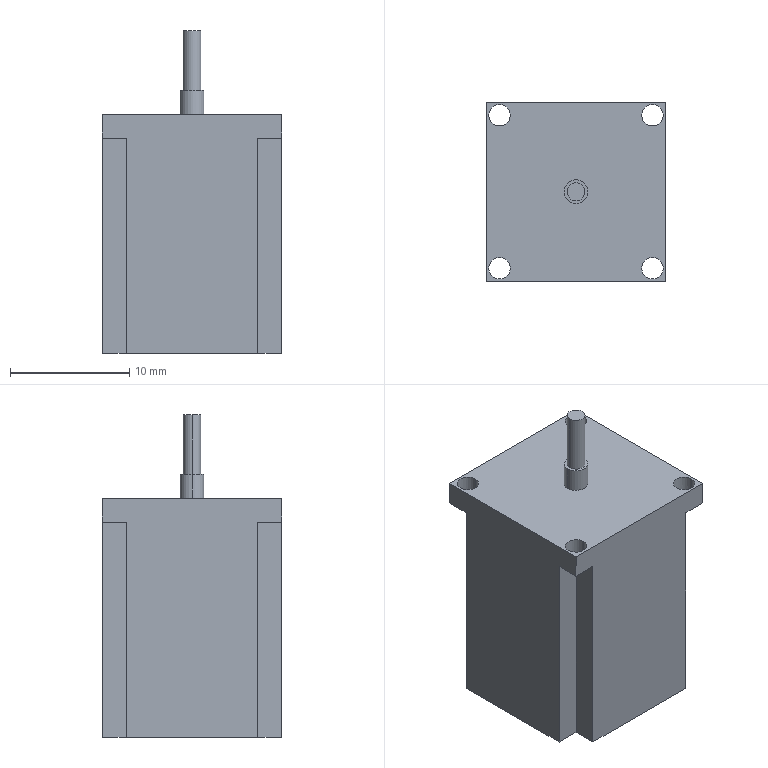Part | SolidWorks | features ICE 4, Extrusion 1 | 1 solid | 36 faces | box 15 x 15 x 27 mm | volume 4207 mm3 | plane 24 | cylinder 12 | commonest cylinder face diameters 1.8 x8 1.5 x2 2 x2
STEP:
#1=CARTESIAN_POINT('',(0.75,0.,27.));
#2=VERTEX_POINT('',#1);
#3=CARTESIAN_POINT('',(-0.75,0.,27.));
#4=VERTEX_POINT('',#3);
#5=CARTESIAN_POINT('',(0.,0.,27.));
#6=DIRECTION('',(0.,0.,1.));
#7=DIRECTION('',(1.,0.,0.));
#8=AXIS2_PLACEMENT_3D('',#5,#6,#7);
#9=CIRCLE('',#8,0.75);
#10=EDGE_CURVE('',#2,#4,#9,.T.);
#11=ORIENTED_EDGE('',*,*,#10,.F.);
#12=CARTESIAN_POINT('',(0.75,0.,22.));
#13=VERTEX_POINT('',#12);
#14=CARTESIAN_POINT('',(0.75,0.,27.));
#15=DIRECTION('',(0.,0.,-1.));
#16=VECTOR('',#15,1000.);
#17=LINE('',#14,#16);
#18=EDGE_CURVE('',#2,#13,#17,.T.);
#19=ORIENTED_EDGE('',*,*,#18,.T.);
#20=CARTESIAN_POINT('',(-0.75,0.,22.));
#21=VERTEX_POINT('',#20);
#22=CARTESIAN_POINT('',(0.,0.,22.));
#23=DIRECTION('',(0.,0.,1.));
#24=DIRECTION('',(1.,0.,0.));
#25=AXIS2_PLACEMENT_3D('',#22,#23,#24);
#26=CIRCLE('',#25,0.75);
#27=EDGE_CURVE('',#13,#21,#26,.T.);
#28=ORIENTED_EDGE('',*,*,#27,.T.);
#29=CARTESIAN_POINT('',(-0.75,0.,27.));
#30=DIRECTION('',(0.,0.,-1.));
#31=VECTOR('',#30,1000.);
#32=LINE('',#29,#31);
#33=EDGE_CURVE('',#4,#21,#32,.T.);
#34=ORIENTED_EDGE('',*,*,#33,.F.);
#35=EDGE_LOOP('',(#11,#19,#28,#34));
#36=FACE_OUTER_BOUND('',#35,.T.);
#37=CARTESIAN_POINT('',(0.,0.,27.));
#38=DIRECTION('',(0.,0.,-1.));
#39=DIRECTION('',(-1.,0.,0.));
#40=AXIS2_PLACEMENT_3D('',#37,#38,#39);
#41=CYLINDRICAL_SURFACE('',#40,0.75);
#42=ADVANCED_FACE('',(#36),#41,.T.);
#43=CARTESIAN_POINT('',(1.,0.,22.));
#44=VERTEX_POINT('',#43);
#45=CARTESIAN_POINT('',(-1.,0.,22.));
#46=VERTEX_POINT('',#45);
#47=CARTESIAN_POINT('',(0.,0.,22.));
#48=DIRECTION('',(0.,0.,1.));
#49=DIRECTION('',(1.,0.,0.));
#50=AXIS2_PLACEMENT_3D('',#47,#48,#49);
#51=CIRCLE('',#50,1.);
#52=EDGE_CURVE('',#44,#46,#51,.T.);
#53=ORIENTED_EDGE('',*,*,#52,.F.);
#54=CARTESIAN_POINT('',(1.,0.,20.));
#55=VERTEX_POINT('',#54);
#56=CARTESIAN_POINT('',(1.,0.,22.));
#57=DIRECTION('',(0.,0.,-1.));
#58=VECTOR('',#57,1000.);
#59=LINE('',#56,#58);
#60=EDGE_CURVE('',#44,#55,#59,.T.);
#61=ORIENTED_EDGE('',*,*,#60,.T.);
#62=CARTESIAN_POINT('',(-1.,0.,20.));
#63=VERTEX_POINT('',#62);
#64=CARTESIAN_POINT('',(0.,0.,20.));
#65=DIRECTION('',(0.,0.,1.));
#66=DIRECTION('',(-1.,0.,0.));
#67=AXIS2_PLACEMENT_3D('',#64,#65,#66);
#68=CIRCLE('',#67,1.);
#69=EDGE_CURVE('',#55,#63,#68,.T.);
#70=ORIENTED_EDGE('',*,*,#69,.T.);
#71=CARTESIAN_POINT('',(-1.,0.,22.));
#72=DIRECTION('',(0.,0.,-1.));
#73=VECTOR('',#72,1000.);
#74=LINE('',#71,#73);
#75=EDGE_CURVE('',#46,#63,#74,.T.);
#76=ORIENTED_EDGE('',*,*,#75,.F.);
#77=EDGE_LOOP('',(#53,#61,#70,#76));
#78=FACE_OUTER_BOUND('',#77,.T.);
#79=CARTESIAN_POINT('',(0.,0.,22.));
#80=DIRECTION('',(0.,0.,-1.));
#81=DIRECTION('',(-1.,0.,0.));
#82=AXIS2_PLACEMENT_3D('',#79,#80,#81);
#83=CYLINDRICAL_SURFACE('',#82,1.);
#84=ADVANCED_FACE('',(#78),#83,.T.);
#85=CARTESIAN_POINT('',(-7.3,6.4,18.));
#86=VERTEX_POINT('',#85);
#87=CARTESIAN_POINT('',(-6.4,5.5,18.));
#88=VERTEX_POINT('',#87);
#89=CARTESIAN_POINT('',(-6.4,6.4,18.));
#90=DIRECTION('',(0.,0.,1.));
#91=DIRECTION('',(1.,0.,0.));
#92=AXIS2_PLACEMENT_3D('',#89,#90,#91);
#93=CIRCLE('',#92,0.9);
#94=EDGE_CURVE('',#86,#88,#93,.T.);
#95=ORIENTED_EDGE('',*,*,#94,.F.);
#96=CARTESIAN_POINT('',(-7.3,6.4,20.));
#97=VERTEX_POINT('',#96);
#98=CARTESIAN_POINT('',(-7.3,6.4,-51.));
#99=DIRECTION('',(0.,0.,1.));
#100=VECTOR('',#99,1000.);
#101=LINE('',#98,#100);
#102=EDGE_CURVE('',#86,#97,#101,.T.);
#103=ORIENTED_EDGE('',*,*,#102,.T.);
#104=CARTESIAN_POINT('',(-5.5,6.4,20.));
#105=VERTEX_POINT('',#104);
#106=CARTESIAN_POINT('',(-6.4,6.4,20.));
#107=DIRECTION('',(0.,0.,1.));
#108=DIRECTION('',(1.,0.,0.));
#109=AXIS2_PLACEMENT_3D('',#106,#107,#108);
#110=CIRCLE('',#109,0.9);
#111=EDGE_CURVE('',#97,#105,#110,.T.);
#112=ORIENTED_EDGE('',*,*,#111,.T.);
#113=CARTESIAN_POINT('',(-5.5,6.4,18.));
#114=VERTEX_POINT('',#113);
#115=CARTESIAN_POINT('',(-5.5,6.4,-51.));
#116=DIRECTION('',(0.,0.,1.));
#117=VECTOR('',#116,1000.);
#118=LINE('',#115,#117);
#119=EDGE_CURVE('',#114,#105,#118,.T.);
#120=ORIENTED_EDGE('',*,*,#119,.F.);
#121=CARTESIAN_POINT('',(-6.4,6.4,18.));
#122=DIRECTION('',(0.,0.,1.));
#123=DIRECTION('',(1.,0.,0.));
#124=AXIS2_PLACEMENT_3D('',#121,#122,#123);
#125=CIRCLE('',#124,0.9);
#126=EDGE_CURVE('',#88,#114,#125,.T.);
#127=ORIENTED_EDGE('',*,*,#126,.F.);
#128=EDGE_LOOP('',(#95,#103,#112,#120,#127));
#129=FACE_OUTER_BOUND('',#128,.T.);
#130=CARTESIAN_POINT('',(-6.4,6.4,-51.));
#131=DIRECTION('',(0.,0.,1.));
#132=DIRECTION('',(1.,0.,0.));
#133=AXIS2_PLACEMENT_3D('',#130,#131,#132);
#134=CYLINDRICAL_SURFACE('',#133,0.9);
#135=ADVANCED_FACE('',(#129),#134,.F.);
#136=CARTESIAN_POINT('',(5.5,-6.4,18.));
#137=VERTEX_POINT('',#136);
#138=CARTESIAN_POINT('',(7.3,-6.4,18.));
#139=VERTEX_POINT('',#138);
#140=CARTESIAN_POINT('',(6.4,-6.4,18.));
#141=DIRECTION('',(0.,0.,1.));
#142=DIRECTION('',(1.,0.,0.));
#143=AXIS2_PLACEMENT_3D('',#140,#141,#142);
#144=CIRCLE('',#143,0.9);
#145=EDGE_CURVE('',#137,#139,#144,.T.);
#146=ORIENTED_EDGE('',*,*,#145,.F.);
#147=CARTESIAN_POINT('',(5.5,-6.4,20.));
#148=VERTEX_POINT('',#147);
#149=CARTESIAN_POINT('',(5.5,-6.4,-51.));
#150=DIRECTION('',(0.,0.,1.));
#151=VECTOR('',#150,1000.);
#152=LINE('',#149,#151);
#153=EDGE_CURVE('',#137,#148,#152,.T.);
#154=ORIENTED_EDGE('',*,*,#153,.T.);
#155=CARTESIAN_POINT('',(7.3,-6.4,20.));
#156=VERTEX_POINT('',#155);
#157=CARTESIAN_POINT('',(6.4,-6.4,20.));
#158=DIRECTION('',(0.,0.,1.));
#159=DIRECTION('',(1.,0.,0.));
#160=AXIS2_PLACEMENT_3D('',#157,#158,#159);
#161=CIRCLE('',#160,0.9);
#162=EDGE_CURVE('',#148,#156,#161,.T.);
#163=ORIENTED_EDGE('',*,*,#162,.T.);
#164=CARTESIAN_POINT('',(7.3,-6.4,-51.));
#165=DIRECTION('',(0.,0.,1.));
#166=VECTOR('',#165,1000.);
#167=LINE('',#164,#166);
#168=EDGE_CURVE('',#139,#156,#167,.T.);
#169=ORIENTED_EDGE('',*,*,#168,.F.);
#170=EDGE_LOOP('',(#146,#154,#163,#169));
#171=FACE_OUTER_BOUND('',#170,.T.);
#172=CARTESIAN_POINT('',(6.4,-6.4,-51.));
#173=DIRECTION('',(0.,0.,1.));
#174=DIRECTION('',(1.,0.,0.));
#175=AXIS2_PLACEMENT_3D('',#172,#173,#174);
#176=CYLINDRICAL_SURFACE('',#175,0.9);
#177=ADVANCED_FACE('',(#171),#176,.F.);
#178=CARTESIAN_POINT('',(-5.5,-6.4,18.));
#179=VERTEX_POINT('',#178);
#180=CARTESIAN_POINT('',(-7.3,-6.4,18.));
#181=VERTEX_POINT('',#180);
#182=CARTESIAN_POINT('',(-6.4,-6.4,18.));
#183=DIRECTION('',(0.,0.,-1.));
#184=DIRECTION('',(-1.,0.,0.));
#185=AXIS2_PLACEMENT_3D('',#182,#183,#184);
#186=CIRCLE('',#185,0.9);
#187=EDGE_CURVE('',#179,#181,#186,.T.);
#188=ORIENTED_EDGE('',*,*,#187,.T.);
#189=CARTESIAN_POINT('',(-7.3,-6.4,20.));
#190=VERTEX_POINT('',#189);
#191=CARTESIAN_POINT('',(-7.3,-6.4,-51.));
#192=DIRECTION('',(0.,0.,1.));
#193=VECTOR('',#192,1000.);
#194=LINE('',#191,#193);
#195=EDGE_CURVE('',#181,#190,#194,.T.);
#196=ORIENTED_EDGE('',*,*,#195,.T.);
#197=CARTESIAN_POINT('',(-5.5,-6.4,20.));
#198=VERTEX_POINT('',#197);
#199=CARTESIAN_POINT('',(-6.4,-6.4,20.));
#200=DIRECTION('',(0.,0.,1.));
#201=DIRECTION('',(1.,0.,0.));
#202=AXIS2_PLACEMENT_3D('',#199,#200,#201);
#203=CIRCLE('',#202,0.9);
#204=EDGE_CURVE('',#190,#198,#203,.T.);
#205=ORIENTED_EDGE('',*,*,#204,.T.);
#206=CARTESIAN_POINT('',(-5.5,-6.4,-51.));
#207=DIRECTION('',(0.,0.,1.));
#208=VECTOR('',#207,1000.);
#209=LINE('',#206,#208);
#210=EDGE_CURVE('',#179,#198,#209,.T.);
#211=ORIENTED_EDGE('',*,*,#210,.F.);
#212=EDGE_LOOP('',(#188,#196,#205,#211));
#213=FACE_OUTER_BOUND('',#212,.T.);
#214=CARTESIAN_POINT('',(-6.4,-6.4,-51.));
#215=DIRECTION('',(0.,0.,1.));
#216=DIRECTION('',(1.,0.,0.));
#217=AXIS2_PLACEMENT_3D('',#214,#215,#216);
#218=CYLINDRICAL_SURFACE('',#217,0.9);
#219=ADVANCED_FACE('',(#213),#218,.F.);
#220=CARTESIAN_POINT('',(6.4,5.5,18.));
#221=VERTEX_POINT('',#220);
#222=CARTESIAN_POINT('',(5.5,6.4,18.));
#223=VERTEX_POINT('',#222);
#224=CARTESIAN_POINT('',(6.4,6.4,18.));
#225=DIRECTION('',(0.,0.,-1.));
#226=DIRECTION('',(-1.,0.,0.));
#227=AXIS2_PLACEMENT_3D('',#224,#225,#226);
#228=CIRCLE('',#227,0.9);
#229=EDGE_CURVE('',#221,#223,#228,.T.);
#230=ORIENTED_EDGE('',*,*,#229,.T.);
#231=CARTESIAN_POINT('',(5.5,6.4,20.));
#232=VERTEX_POINT('',#231);
#233=CARTESIAN_POINT('',(5.5,6.4,-51.));
#234=DIRECTION('',(0.,0.,1.));
#235=VECTOR('',#234,1000.);
#236=LINE('',#233,#235);
#237=EDGE_CURVE('',#223,#232,#236,.T.);
#238=ORIENTED_EDGE('',*,*,#237,.T.);
#239=CARTESIAN_POINT('',(7.3,6.4,20.));
#240=VERTEX_POINT('',#239);
#241=CARTESIAN_POINT('',(6.4,6.4,20.));
#242=DIRECTION('',(0.,0.,1.));
#243=DIRECTION('',(1.,0.,0.));
#244=AXIS2_PLACEMENT_3D('',#241,#242,#243);
#245=CIRCLE('',#244,0.9);
#246=EDGE_CURVE('',#232,#240,#245,.T.);
#247=ORIENTED_EDGE('',*,*,#246,.T.);
#248=CARTESIAN_POINT('',(7.3,6.4,18.));
#249=VERTEX_POINT('',#248);
#250=CARTESIAN_POINT('',(7.3,6.4,-51.));
#251=DIRECTION('',(0.,0.,1.));
#252=VECTOR('',#251,1000.);
#253=LINE('',#250,#252);
#254=EDGE_CURVE('',#249,#240,#253,.T.);
#255=ORIENTED_EDGE('',*,*,#254,.F.);
#256=CARTESIAN_POINT('',(6.4,6.4,18.));
#257=DIRECTION('',(0.,0.,-1.));
#258=DIRECTION('',(-1.,0.,0.));
#259=AXIS2_PLACEMENT_3D('',#256,#257,#258);
#260=CIRCLE('',#259,0.9);
#261=EDGE_CURVE('',#249,#221,#260,.T.);
#262=ORIENTED_EDGE('',*,*,#261,.T.);
#263=EDGE_LOOP('',(#230,#238,#247,#255,#262));
#264=FACE_OUTER_BOUND('',#263,.T.);
#265=CARTESIAN_POINT('',(6.4,6.4,-51.));
#266=DIRECTION('',(0.,0.,1.));
#267=DIRECTION('',(1.,0.,0.));
#268=AXIS2_PLACEMENT_3D('',#265,#266,#267);
#269=CYLINDRICAL_SURFACE('',#268,0.9);
#270=ADVANCED_FACE('',(#264),#269,.F.);
#271=CARTESIAN_POINT('',(-5.5,7.5,18.));
#272=VERTEX_POINT('',#271);
#273=CARTESIAN_POINT('',(-5.5,7.5,18.));
#274=DIRECTION('',(0.,-1.,0.));
#275=VECTOR('',#274,1000.);
#276=LINE('',#273,#275);
#277=EDGE_CURVE('',#272,#114,#276,.T.);
#278=ORIENTED_EDGE('',*,*,#277,.T.);
#279=CARTESIAN_POINT('',(-6.4,6.4,18.));
#280=DIRECTION('',(0.,0.,1.));
#281=DIRECTION('',(1.,0.,0.));
#282=AXIS2_PLACEMENT_3D('',#279,#280,#281);
#283=CIRCLE('',#282,0.9);
#284=EDGE_CURVE('',#114,#86,#283,.T.);
#285=ORIENTED_EDGE('',*,*,#284,.T.);
#286=ORIENTED_EDGE('',*,*,#94,.T.);
#287=CARTESIAN_POINT('',(-7.5,5.5,18.));
#288=VERTEX_POINT('',#287);
#289=CARTESIAN_POINT('',(-7.5,5.5,18.));
#290=DIRECTION('',(-1.,0.,0.));
#291=VECTOR('',#290,1000.);
#292=LINE('',#289,#291);
#293=EDGE_CURVE('',#88,#288,#292,.T.);
#294=ORIENTED_EDGE('',*,*,#293,.T.);
#295=CARTESIAN_POINT('',(-7.5,7.5,18.));
#296=VERTEX_POINT('',#295);
#297=CARTESIAN_POINT('',(-7.5,7.5,18.));
#298=DIRECTION('',(0.,1.,0.));
#299=VECTOR('',#298,1000.);
#300=LINE('',#297,#299);
#301=EDGE_CURVE('',#288,#296,#300,.T.);
#302=ORIENTED_EDGE('',*,*,#301,.T.);
#303=CARTESIAN_POINT('',(-7.5,7.5,18.));
#304=DIRECTION('',(1.,0.,0.));
#305=VECTOR('',#304,1000.);
#306=LINE('',#303,#305);
#307=EDGE_CURVE('',#296,#272,#306,.T.);
#308=ORIENTED_EDGE('',*,*,#307,.T.);
#309=EDGE_LOOP('',(#278,#285,#286,#294,#302,#308));
#310=FACE_OUTER_BOUND('',#309,.T.);
#311=CARTESIAN_POINT('',(0.,0.,18.));
#312=DIRECTION('',(0.,0.,1.));
#313=DIRECTION('',(1.,0.,0.));
#314=AXIS2_PLACEMENT_3D('',#311,#312,#313);
#315=PLANE('',#314);
#316=ADVANCED_FACE('',(#310),#315,.F.);
#317=CARTESIAN_POINT('',(5.5,-5.5,18.));
#318=VERTEX_POINT('',#317);
#319=CARTESIAN_POINT('',(6.4,-5.5,18.));
#320=VERTEX_POINT('',#319);
#321=CARTESIAN_POINT('',(7.5,-5.5,18.));
#322=DIRECTION('',(1.,0.,0.));
#323=VECTOR('',#322,1000.);
#324=LINE('',#321,#323);
#325=EDGE_CURVE('',#318,#320,#324,.T.);
#326=ORIENTED_EDGE('',*,*,#325,.T.);
#327=CARTESIAN_POINT('',(6.4,-6.4,18.));
#328=DIRECTION('',(0.,0.,1.));
#329=DIRECTION('',(1.,0.,0.));
#330=AXIS2_PLACEMENT_3D('',#327,#328,#329);
#331=CIRCLE('',#330,0.9);
#332=EDGE_CURVE('',#320,#137,#331,.T.);
#333=ORIENTED_EDGE('',*,*,#332,.T.);
#334=CARTESIAN_POINT('',(5.5,-7.5,18.));
#335=DIRECTION('',(0.,1.,0.));
#336=VECTOR('',#335,1000.);
#337=LINE('',#334,#336);
#338=EDGE_CURVE('',#137,#318,#337,.T.);
#339=ORIENTED_EDGE('',*,*,#338,.T.);
#340=EDGE_LOOP('',(#326,#333,#339));
#341=FACE_OUTER_BOUND('',#340,.T.);
#342=CARTESIAN_POINT('',(0.,0.,18.));
#343=DIRECTION('',(0.,0.,1.));
#344=DIRECTION('',(1.,0.,0.));
#345=AXIS2_PLACEMENT_3D('',#342,#343,#344);
#346=PLANE('',#345);
#347=ADVANCED_FACE('',(#341),#346,.F.);
#348=CARTESIAN_POINT('',(-6.4,-5.5,18.));
#349=VERTEX_POINT('',#348);
#350=CARTESIAN_POINT('',(-6.4,-6.4,18.));
#351=DIRECTION('',(0.,0.,-1.));
#352=DIRECTION('',(-1.,0.,0.));
#353=AXIS2_PLACEMENT_3D('',#350,#351,#352);
#354=CIRCLE('',#353,0.9);
#355=EDGE_CURVE('',#349,#179,#354,.T.);
#356=ORIENTED_EDGE('',*,*,#355,.F.);
#357=CARTESIAN_POINT('',(-5.5,-5.5,18.));
#358=VERTEX_POINT('',#357);
#359=CARTESIAN_POINT('',(-7.5,-5.5,18.));
#360=DIRECTION('',(1.,0.,0.));
#361=VECTOR('',#360,1000.);
#362=LINE('',#359,#361);
#363=EDGE_CURVE('',#349,#358,#362,.T.);
#364=ORIENTED_EDGE('',*,*,#363,.T.);
#365=CARTESIAN_POINT('',(-5.5,-7.5,18.));
#366=DIRECTION('',(0.,-1.,0.));
#367=VECTOR('',#366,1000.);
#368=LINE('',#365,#367);
#369=EDGE_CURVE('',#358,#179,#368,.T.);
#370=ORIENTED_EDGE('',*,*,#369,.T.);
#371=EDGE_LOOP('',(#356,#364,#370));
#372=FACE_OUTER_BOUND('',#371,.T.);
#373=CARTESIAN_POINT('',(0.,0.,18.));
#374=DIRECTION('',(0.,0.,-1.));
#375=DIRECTION('',(-1.,0.,0.));
#376=AXIS2_PLACEMENT_3D('',#373,#374,#375);
#377=PLANE('',#376);
#378=ADVANCED_FACE('',(#372),#377,.T.);
#379=CARTESIAN_POINT('',(6.4,6.4,18.));
#380=DIRECTION('',(0.,0.,-1.));
#381=DIRECTION('',(-1.,0.,0.));
#382=AXIS2_PLACEMENT_3D('',#379,#380,#381);
#383=CIRCLE('',#382,0.9);
#384=EDGE_CURVE('',#223,#249,#383,.T.);
#385=ORIENTED_EDGE('',*,*,#384,.F.);
#386=CARTESIAN_POINT('',(5.5,7.5,18.));
#387=VERTEX_POINT('',#386);
#388=CARTESIAN_POINT('',(5.5,7.5,18.));
#389=DIRECTION('',(0.,1.,0.));
#390=VECTOR('',#389,1000.);
#391=LINE('',#388,#390);
#392=EDGE_CURVE('',#223,#387,#391,.T.);
#393=ORIENTED_EDGE('',*,*,#392,.T.);
#394=CARTESIAN_POINT('',(7.5,7.5,18.));
#395=VERTEX_POINT('',#394);
#396=CARTESIAN_POINT('',(7.5,7.5,18.));
#397=DIRECTION('',(1.,0.,0.));
#398=VECTOR('',#397,1000.);
#399=LINE('',#396,#398);
#400=EDGE_CURVE('',#387,#395,#399,.T.);
#401=ORIENTED_EDGE('',*,*,#400,.T.);
#402=CARTESIAN_POINT('',(7.5,5.5,18.));
#403=VERTEX_POINT('',#402);
#404=CARTESIAN_POINT('',(7.5,7.5,18.));
#405=DIRECTION('',(0.,-1.,0.));
#406=VECTOR('',#405,1000.);
#407=LINE('',#404,#406);
#408=EDGE_CURVE('',#395,#403,#407,.T.);
#409=ORIENTED_EDGE('',*,*,#408,.T.);
#410=CARTESIAN_POINT('',(7.5,5.5,18.));
#411=DIRECTION('',(-1.,0.,0.));
#412=VECTOR('',#411,1000.);
#413=LINE('',#410,#412);
#414=EDGE_CURVE('',#403,#221,#413,.T.);
#415=ORIENTED_EDGE('',*,*,#414,.T.);
#416=ORIENTED_EDGE('',*,*,#261,.F.);
#417=EDGE_LOOP('',(#385,#393,#401,#409,#415,#416));
#418=FACE_OUTER_BOUND('',#417,.T.);
#419=CARTESIAN_POINT('',(0.,0.,18.));
#420=DIRECTION('',(0.,0.,-1.));
#421=DIRECTION('',(-1.,0.,0.));
#422=AXIS2_PLACEMENT_3D('',#419,#420,#421);
#423=PLANE('',#422);
#424=ADVANCED_FACE('',(#418),#423,.T.);
#425=CARTESIAN_POINT('',(7.5,-5.5,18.));
#426=VERTEX_POINT('',#425);
#427=CARTESIAN_POINT('',(7.5,-7.5,18.));
#428=VERTEX_POINT('',#427);
#429=CARTESIAN_POINT('',(7.5,-7.5,18.));
#430=DIRECTION('',(0.,-1.,0.));
#431=VECTOR('',#430,1000.);
#432=LINE('',#429,#431);
#433=EDGE_CURVE('',#426,#428,#432,.T.);
#434=ORIENTED_EDGE('',*,*,#433,.F.);
#435=CARTESIAN_POINT('',(7.5,-5.5,0.));
#436=VERTEX_POINT('',#435);
#437=CARTESIAN_POINT('',(7.5,-5.5,18.));
#438=DIRECTION('',(0.,0.,-1.));
#439=VECTOR('',#438,1000.);
#440=LINE('',#437,#439);
#441=EDGE_CURVE('',#426,#436,#440,.T.);
#442=ORIENTED_EDGE('',*,*,#441,.T.);
#443=CARTESIAN_POINT('',(7.5,5.5,0.));
#444=VERTEX_POINT('',#443);
#445=CARTESIAN_POINT('',(7.5,-7.5,0.));
#446=DIRECTION('',(0.,1.,0.));
#447=VECTOR('',#446,1000.);
#448=LINE('',#445,#447);
#449=EDGE_CURVE('',#436,#444,#448,.T.);
#450=ORIENTED_EDGE('',*,*,#449,.T.);
#451=CARTESIAN_POINT('',(7.5,5.5,18.));
#452=DIRECTION('',(0.,0.,-1.));
#453=VECTOR('',#452,1000.);
#454=LINE('',#451,#453);
#455=EDGE_CURVE('',#403,#444,#454,.T.);
#456=ORIENTED_EDGE('',*,*,#455,.F.);
#457=ORIENTED_EDGE('',*,*,#408,.F.);
#458=CARTESIAN_POINT('',(7.5,7.5,20.));
#459=VERTEX_POINT('',#458);
#460=CARTESIAN_POINT('',(7.5,7.5,20.));
#461=DIRECTION('',(0.,0.,-1.));
#462=VECTOR('',#461,1000.);
#463=LINE('',#460,#462);
#464=EDGE_CURVE('',#459,#395,#463,.T.);
#465=ORIENTED_EDGE('',*,*,#464,.F.);
#466=CARTESIAN_POINT('',(7.5,-7.5,20.));
#467=VERTEX_POINT('',#466);
#468=CARTESIAN_POINT('',(7.5,-7.5,20.));
#469=DIRECTION('',(0.,1.,0.));
#470=VECTOR('',#469,1000.);
#471=LINE('',#468,#470);
#472=EDGE_CURVE('',#467,#459,#471,.T.);
#473=ORIENTED_EDGE('',*,*,#472,.F.);
#474=CARTESIAN_POINT('',(7.5,-7.5,20.));
#475=DIRECTION('',(0.,0.,-1.));
#476=VECTOR('',#475,1000.);
#477=LINE('',#474,#476);
#478=EDGE_CURVE('',#467,#428,#477,.T.);
#479=ORIENTED_EDGE('',*,*,#478,.T.);
#480=EDGE_LOOP('',(#434,#442,#450,#456,#457,#465,#473,#479));
#481=FACE_OUTER_BOUND('',#480,.T.);
#482=CARTESIAN_POINT('',(7.5,-7.5,20.));
#483=DIRECTION('',(-1.,0.,0.));
#484=DIRECTION('',(0.,0.,1.));
#485=AXIS2_PLACEMENT_3D('',#482,#483,#484);
#486=PLANE('',#485);
#487=ADVANCED_FACE('',(#481),#486,.F.);
#488=ORIENTED_EDGE('',*,*,#400,.F.);
#489=CARTESIAN_POINT('',(5.5,7.5,0.));
#490=VERTEX_POINT('',#489);
#491=CARTESIAN_POINT('',(5.5,7.5,18.));
#492=DIRECTION('',(0.,0.,-1.));
#493=VECTOR('',#492,1000.);
#494=LINE('',#491,#493);
#495=EDGE_CURVE('',#387,#490,#494,.T.);
#496=ORIENTED_EDGE('',*,*,#495,.T.);
#497=CARTESIAN_POINT('',(-5.5,7.5,0.));
#498=VERTEX_POINT('',#497);
#499=CARTESIAN_POINT('',(-7.5,7.5,0.));
#500=DIRECTION('',(-1.,0.,0.));
#501=VECTOR('',#500,1000.);
#502=LINE('',#499,#501);
#503=EDGE_CURVE('',#490,#498,#502,.T.);
#504=ORIENTED_EDGE('',*,*,#503,.T.);
#505=CARTESIAN_POINT('',(-5.5,7.5,18.));
#506=DIRECTION('',(0.,0.,-1.));
#507=VECTOR('',#506,1000.);
#508=LINE('',#505,#507);
#509=EDGE_CURVE('',#272,#498,#508,.T.);
#510=ORIENTED_EDGE('',*,*,#509,.F.);
#511=ORIENTED_EDGE('',*,*,#307,.F.);
#512=CARTESIAN_POINT('',(-7.5,7.5,20.));
#513=VERTEX_POINT('',#512);
#514=CARTESIAN_POINT('',(-7.5,7.5,20.));
#515=DIRECTION('',(0.,0.,-1.));
#516=VECTOR('',#515,1000.);
#517=LINE('',#514,#516);
#518=EDGE_CURVE('',#513,#296,#517,.T.);
#519=ORIENTED_EDGE('',*,*,#518,.F.);
#520=CARTESIAN_POINT('',(-7.5,7.5,20.));
#521=DIRECTION('',(-1.,0.,0.));
#522=VECTOR('',#521,1000.);
#523=LINE('',#520,#522);
#524=EDGE_CURVE('',#459,#513,#523,.T.);
#525=ORIENTED_EDGE('',*,*,#524,.F.);
#526=ORIENTED_EDGE('',*,*,#464,.T.);
#527=EDGE_LOOP('',(#488,#496,#504,#510,#511,#519,#525,#526));
#528=FACE_OUTER_BOUND('',#527,.T.);
#529=CARTESIAN_POINT('',(-7.5,7.5,20.));
#530=DIRECTION('',(0.,-1.,0.));
#531=DIRECTION('',(0.,0.,-1.));
#532=AXIS2_PLACEMENT_3D('',#529,#530,#531);
#533=PLANE('',#532);
#534=ADVANCED_FACE('',(#528),#533,.F.);
#535=CARTESIAN_POINT('',(-7.5,5.5,0.));
#536=VERTEX_POINT('',#535);
#537=CARTESIAN_POINT('',(-7.5,-5.5,0.));
#538=VERTEX_POINT('',#537);
#539=CARTESIAN_POINT('',(-7.5,-7.5,0.));
#540=DIRECTION('',(0.,-1.,0.));
#541=VECTOR('',#540,1000.);
#542=LINE('',#539,#541);
#543=EDGE_CURVE('',#536,#538,#542,.T.);
#544=ORIENTED_EDGE('',*,*,#543,.T.);
#545=CARTESIAN_POINT('',(-7.5,-5.5,18.));
#546=VERTEX_POINT('',#545);
#547=CARTESIAN_POINT('',(-7.5,-5.5,18.));
#548=DIRECTION('',(0.,0.,-1.));
#549=VECTOR('',#548,1000.);
#550=LINE('',#547,#549);
#551=EDGE_CURVE('',#546,#538,#550,.T.);
#552=ORIENTED_EDGE('',*,*,#551,.F.);
#553=CARTESIAN_POINT('',(-7.5,-7.5,18.));
#554=VERTEX_POINT('',#553);
#555=CARTESIAN_POINT('',(-7.5,-7.5,18.));
#556=DIRECTION('',(0.,1.,0.));
#557=VECTOR('',#556,1000.);
#558=LINE('',#555,#557);
#559=EDGE_CURVE('',#554,#546,#558,.T.);
#560=ORIENTED_EDGE('',*,*,#559,.F.);
#561=CARTESIAN_POINT('',(-7.5,-7.5,20.));
#562=VERTEX_POINT('',#561);
#563=CARTESIAN_POINT('',(-7.5,-7.5,20.));
#564=DIRECTION('',(0.,0.,-1.));
#565=VECTOR('',#564,1000.);
#566=LINE('',#563,#565);
#567=EDGE_CURVE('',#562,#554,#566,.T.);
#568=ORIENTED_EDGE('',*,*,#567,.F.);
#569=CARTESIAN_POINT('',(-7.5,-7.5,20.));
#570=DIRECTION('',(0.,-1.,0.));
#571=VECTOR('',#570,1000.);
#572=LINE('',#569,#571);
#573=EDGE_CURVE('',#513,#562,#572,.T.);
#574=ORIENTED_EDGE('',*,*,#573,.F.);
#575=ORIENTED_EDGE('',*,*,#518,.T.);
#576=ORIENTED_EDGE('',*,*,#301,.F.);
#577=CARTESIAN_POINT('',(-7.5,5.5,18.));
#578=DIRECTION('',(0.,0.,-1.));
#579=VECTOR('',#578,1000.);
#580=LINE('',#577,#579);
#581=EDGE_CURVE('',#288,#536,#580,.T.);
#582=ORIENTED_EDGE('',*,*,#581,.T.);
#583=EDGE_LOOP('',(#544,#552,#560,#568,#574,#575,#576,#582));
#584=FACE_OUTER_BOUND('',#583,.T.);
#585=CARTESIAN_POINT('',(-7.5,-7.5,20.));
#586=DIRECTION('',(1.,0.,0.));
#587=DIRECTION('',(0.,0.,-1.));
#588=AXIS2_PLACEMENT_3D('',#585,#586,#587);
#589=PLANE('',#588);
#590=ADVANCED_FACE('',(#584),#589,.F.);
#591=CARTESIAN_POINT('',(-5.5,-7.5,18.));
#592=VERTEX_POINT('',#591);
#593=CARTESIAN_POINT('',(-7.5,-7.5,18.));
#594=DIRECTION('',(-1.,0.,0.));
#595=VECTOR('',#594,1000.);
#596=LINE('',#593,#595);
#597=EDGE_CURVE('',#592,#554,#596,.T.);
#598=ORIENTED_EDGE('',*,*,#597,.F.);
#599=CARTESIAN_POINT('',(-5.5,-7.5,0.));
#600=VERTEX_POINT('',#599);
#601=CARTESIAN_POINT('',(-5.5,-7.5,18.));
#602=DIRECTION('',(0.,0.,-1.));
#603=VECTOR('',#602,1000.);
#604=LINE('',#601,#603);
#605=EDGE_CURVE('',#592,#600,#604,.T.);
#606=ORIENTED_EDGE('',*,*,#605,.T.);
#607=CARTESIAN_POINT('',(5.5,-7.5,0.));
#608=VERTEX_POINT('',#607);
#609=CARTESIAN_POINT('',(-7.5,-7.5,0.));
#610=DIRECTION('',(1.,0.,0.));
#611=VECTOR('',#610,1000.);
#612=LINE('',#609,#611);
#613=EDGE_CURVE('',#600,#608,#612,.T.);
#614=ORIENTED_EDGE('',*,*,#613,.T.);
#615=CARTESIAN_POINT('',(5.5,-7.5,18.));
#616=VERTEX_POINT('',#615);
#617=CARTESIAN_POINT('',(5.5,-7.5,18.));
#618=DIRECTION('',(0.,0.,-1.));
#619=VECTOR('',#618,1000.);
#620=LINE('',#617,#619);
#621=EDGE_CURVE('',#616,#608,#620,.T.);
#622=ORIENTED_EDGE('',*,*,#621,.F.);
#623=CARTESIAN_POINT('',(7.5,-7.5,18.));
#624=DIRECTION('',(-1.,0.,0.));
#625=VECTOR('',#624,1000.);
#626=LINE('',#623,#625);
#627=EDGE_CURVE('',#428,#616,#626,.T.);
#628=ORIENTED_EDGE('',*,*,#627,.F.);
#629=ORIENTED_EDGE('',*,*,#478,.F.);
#630=CARTESIAN_POINT('',(-7.5,-7.5,20.));
#631=DIRECTION('',(1.,0.,0.));
#632=VECTOR('',#631,1000.);
#633=LINE('',#630,#632);
#634=EDGE_CURVE('',#562,#467,#633,.T.);
#635=ORIENTED_EDGE('',*,*,#634,.F.);
#636=ORIENTED_EDGE('',*,*,#567,.T.);
#637=EDGE_LOOP('',(#598,#606,#614,#622,#628,#629,#635,#636));
#638=FACE_OUTER_BOUND('',#637,.T.);
#639=CARTESIAN_POINT('',(-7.5,-7.5,20.));
#640=DIRECTION('',(0.,1.,0.));
#641=DIRECTION('',(0.,0.,1.));
#642=AXIS2_PLACEMENT_3D('',#639,#640,#641);
#643=PLANE('',#642);
#644=ADVANCED_FACE('',(#638),#643,.F.);
#645=CARTESIAN_POINT('',(0.,0.,20.));
#646=DIRECTION('',(0.,0.,1.));
#647=DIRECTION('',(-1.,0.,0.));
#648=AXIS2_PLACEMENT_3D('',#645,#646,#647);
#649=CIRCLE('',#648,1.);
#650=EDGE_CURVE('',#63,#55,#649,.T.);
#651=ORIENTED_EDGE('',*,*,#650,.F.);
#652=ORIENTED_EDGE('',*,*,#69,.F.);
#653=EDGE_LOOP('',(#651,#652));
#654=FACE_BOUND('',#653,.T.);
#655=CARTESIAN_POINT('',(-6.4,6.4,20.));
#656=DIRECTION('',(0.,0.,1.));
#657=DIRECTION('',(1.,0.,0.));
#658=AXIS2_PLACEMENT_3D('',#655,#656,#657);
#659=CIRCLE('',#658,0.9);
#660=EDGE_CURVE('',#105,#97,#659,.T.);
#661=ORIENTED_EDGE('',*,*,#660,.F.);
#662=ORIENTED_EDGE('',*,*,#111,.F.);
#663=EDGE_LOOP('',(#661,#662));
#664=FACE_BOUND('',#663,.T.);
#665=CARTESIAN_POINT('',(-6.4,-6.4,20.));
#666=DIRECTION('',(0.,0.,1.));
#667=DIRECTION('',(1.,0.,0.));
#668=AXIS2_PLACEMENT_3D('',#665,#666,#667);
#669=CIRCLE('',#668,0.9);
#670=EDGE_CURVE('',#198,#190,#669,.T.);
#671=ORIENTED_EDGE('',*,*,#670,.F.);
#672=ORIENTED_EDGE('',*,*,#204,.F.);
#673=EDGE_LOOP('',(#671,#672));
#674=FACE_BOUND('',#673,.T.);
#675=CARTESIAN_POINT('',(6.4,-6.4,20.));
#676=DIRECTION('',(0.,0.,1.));
#677=DIRECTION('',(1.,0.,0.));
#678=AXIS2_PLACEMENT_3D('',#675,#676,#677);
#679=CIRCLE('',#678,0.9);
#680=EDGE_CURVE('',#156,#148,#679,.T.);
#681=ORIENTED_EDGE('',*,*,#680,.F.);
#682=ORIENTED_EDGE('',*,*,#162,.F.);
#683=EDGE_LOOP('',(#681,#682));
#684=FACE_BOUND('',#683,.T.);
#685=CARTESIAN_POINT('',(6.4,6.4,20.));
#686=DIRECTION('',(0.,0.,1.));
#687=DIRECTION('',(1.,0.,0.));
#688=AXIS2_PLACEMENT_3D('',#685,#686,#687);
#689=CIRCLE('',#688,0.9);
#690=EDGE_CURVE('',#240,#232,#689,.T.);
#691=ORIENTED_EDGE('',*,*,#690,.F.);
#692=ORIENTED_EDGE('',*,*,#246,.F.);
#693=EDGE_LOOP('',(#691,#692));
#694=FACE_BOUND('',#693,.T.);
#695=ORIENTED_EDGE('',*,*,#472,.T.);
#696=ORIENTED_EDGE('',*,*,#524,.T.);
#697=ORIENTED_EDGE('',*,*,#573,.T.);
#698=ORIENTED_EDGE('',*,*,#634,.T.);
#699=EDGE_LOOP('',(#695,#696,#697,#698));
#700=FACE_OUTER_BOUND('',#699,.T.);
#701=CARTESIAN_POINT('',(0.,0.,20.));
#702=DIRECTION('',(0.,0.,-1.));
#703=DIRECTION('',(-1.,0.,0.));
#704=AXIS2_PLACEMENT_3D('',#701,#702,#703);
#705=PLANE('',#704);
#706=ADVANCED_FACE('',(#654,#664,#674,#684,#694,#700),#705,.F.);
#707=CARTESIAN_POINT('',(-5.5,-5.5,0.));
#708=VERTEX_POINT('',#707);
#709=CARTESIAN_POINT('',(-5.5,-7.5,0.));
#710=DIRECTION('',(0.,-1.,0.));
#711=VECTOR('',#710,1000.);
#712=LINE('',#709,#711);
#713=EDGE_CURVE('',#708,#600,#712,.T.);
#714=ORIENTED_EDGE('',*,*,#713,.F.);
#715=CARTESIAN_POINT('',(-7.5,-5.5,0.));
#716=DIRECTION('',(1.,0.,0.));
#717=VECTOR('',#716,1000.);
#718=LINE('',#715,#717);
#719=EDGE_CURVE('',#538,#708,#718,.T.);
#720=ORIENTED_EDGE('',*,*,#719,.F.);
#721=ORIENTED_EDGE('',*,*,#543,.F.);
#722=CARTESIAN_POINT('',(-5.5,5.5,0.));
#723=VERTEX_POINT('',#722);
#724=CARTESIAN_POINT('',(-7.5,5.5,0.));
#725=DIRECTION('',(-1.,0.,0.));
#726=VECTOR('',#725,1000.);
#727=LINE('',#724,#726);
#728=EDGE_CURVE('',#723,#536,#727,.T.);
#729=ORIENTED_EDGE('',*,*,#728,.F.);
#730=CARTESIAN_POINT('',(-5.5,7.5,0.));
#731=DIRECTION('',(0.,-1.,0.));
#732=VECTOR('',#731,1000.);
#733=LINE('',#730,#732);
#734=EDGE_CURVE('',#498,#723,#733,.T.);
#735=ORIENTED_EDGE('',*,*,#734,.F.);
#736=ORIENTED_EDGE('',*,*,#503,.F.);
#737=CARTESIAN_POINT('',(5.5,5.5,0.));
#738=VERTEX_POINT('',#737);
#739=CARTESIAN_POINT('',(5.5,7.5,0.));
#740=DIRECTION('',(0.,1.,0.));
#741=VECTOR('',#740,1000.);
#742=LINE('',#739,#741);
#743=EDGE_CURVE('',#738,#490,#742,.T.);
#744=ORIENTED_EDGE('',*,*,#743,.F.);
#745=CARTESIAN_POINT('',(7.5,5.5,0.));
#746=DIRECTION('',(-1.,0.,0.));
#747=VECTOR('',#746,1000.);
#748=LINE('',#745,#747);
#749=EDGE_CURVE('',#444,#738,#748,.T.);
#750=ORIENTED_EDGE('',*,*,#749,.F.);
#751=ORIENTED_EDGE('',*,*,#449,.F.);
#752=CARTESIAN_POINT('',(5.5,-5.5,0.));
#753=VERTEX_POINT('',#752);
#754=CARTESIAN_POINT('',(7.5,-5.5,0.));
#755=DIRECTION('',(1.,0.,0.));
#756=VECTOR('',#755,1000.);
#757=LINE('',#754,#756);
#758=EDGE_CURVE('',#753,#436,#757,.T.);
#759=ORIENTED_EDGE('',*,*,#758,.F.);
#760=CARTESIAN_POINT('',(5.5,-7.5,0.));
#761=DIRECTION('',(0.,1.,0.));
#762=VECTOR('',#761,1000.);
#763=LINE('',#760,#762);
#764=EDGE_CURVE('',#608,#753,#763,.T.);
#765=ORIENTED_EDGE('',*,*,#764,.F.);
#766=ORIENTED_EDGE('',*,*,#613,.F.);
#767=EDGE_LOOP('',(#714,#720,#721,#729,#735,#736,#744,#750,#751,#759,#765,#766));
#768=FACE_OUTER_BOUND('',#767,.T.);
#769=CARTESIAN_POINT('',(0.,0.,0.));
#770=DIRECTION('',(0.,0.,-1.));
#771=DIRECTION('',(-1.,0.,0.));
#772=AXIS2_PLACEMENT_3D('',#769,#770,#771);
#773=PLANE('',#772);
#774=ADVANCED_FACE('',(#768),#773,.T.);
#775=ORIENTED_EDGE('',*,*,#728,.T.);
#776=ORIENTED_EDGE('',*,*,#581,.F.);
#777=ORIENTED_EDGE('',*,*,#293,.F.);
#778=CARTESIAN_POINT('',(-5.5,5.5,18.));
#779=VERTEX_POINT('',#778);
#780=CARTESIAN_POINT('',(-7.5,5.5,18.));
#781=DIRECTION('',(-1.,0.,0.));
#782=VECTOR('',#781,1000.);
#783=LINE('',#780,#782);
#784=EDGE_CURVE('',#779,#88,#783,.T.);
#785=ORIENTED_EDGE('',*,*,#784,.F.);
#786=CARTESIAN_POINT('',(-5.5,5.5,18.));
#787=DIRECTION('',(0.,0.,-1.));
#788=VECTOR('',#787,1000.);
#789=LINE('',#786,#788);
#790=EDGE_CURVE('',#779,#723,#789,.T.);
#791=ORIENTED_EDGE('',*,*,#790,.T.);
#792=EDGE_LOOP('',(#775,#776,#777,#785,#791));
#793=FACE_OUTER_BOUND('',#792,.T.);
#794=CARTESIAN_POINT('',(-7.5,5.5,18.));
#795=DIRECTION('',(0.,-1.,0.));
#796=DIRECTION('',(0.,0.,-1.));
#797=AXIS2_PLACEMENT_3D('',#794,#795,#796);
#798=PLANE('',#797);
#799=ADVANCED_FACE('',(#793),#798,.F.);
#800=ORIENTED_EDGE('',*,*,#734,.T.);
#801=ORIENTED_EDGE('',*,*,#790,.F.);
#802=CARTESIAN_POINT('',(-5.5,7.5,18.));
#803=DIRECTION('',(0.,-1.,0.));
#804=VECTOR('',#803,1000.);
#805=LINE('',#802,#804);
#806=EDGE_CURVE('',#114,#779,#805,.T.);
#807=ORIENTED_EDGE('',*,*,#806,.F.);
#808=ORIENTED_EDGE('',*,*,#277,.F.);
#809=ORIENTED_EDGE('',*,*,#509,.T.);
#810=EDGE_LOOP('',(#800,#801,#807,#808,#809));
#811=FACE_OUTER_BOUND('',#810,.T.);
#812=CARTESIAN_POINT('',(-5.5,7.5,18.));
#813=DIRECTION('',(1.,0.,0.));
#814=DIRECTION('',(0.,0.,-1.));
#815=AXIS2_PLACEMENT_3D('',#812,#813,#814);
#816=PLANE('',#815);
#817=ADVANCED_FACE('',(#811),#816,.F.);
#818=ORIENTED_EDGE('',*,*,#784,.T.);
#819=ORIENTED_EDGE('',*,*,#126,.T.);
#820=ORIENTED_EDGE('',*,*,#806,.T.);
#821=EDGE_LOOP('',(#818,#819,#820));
#822=FACE_OUTER_BOUND('',#821,.T.);
#823=CARTESIAN_POINT('',(0.,0.,18.));
#824=DIRECTION('',(0.,0.,1.));
#825=DIRECTION('',(1.,0.,0.));
#826=AXIS2_PLACEMENT_3D('',#823,#824,#825);
#827=PLANE('',#826);
#828=ADVANCED_FACE('',(#822),#827,.F.);
#829=ORIENTED_EDGE('',*,*,#743,.T.);
#830=ORIENTED_EDGE('',*,*,#495,.F.);
#831=ORIENTED_EDGE('',*,*,#392,.F.);
#832=CARTESIAN_POINT('',(5.5,5.5,18.));
#833=VERTEX_POINT('',#832);
#834=CARTESIAN_POINT('',(5.5,7.5,18.));
#835=DIRECTION('',(0.,1.,0.));
#836=VECTOR('',#835,1000.);
#837=LINE('',#834,#836);
#838=EDGE_CURVE('',#833,#223,#837,.T.);
#839=ORIENTED_EDGE('',*,*,#838,.F.);
#840=CARTESIAN_POINT('',(5.5,5.5,18.));
#841=DIRECTION('',(0.,0.,-1.));
#842=VECTOR('',#841,1000.);
#843=LINE('',#840,#842);
#844=EDGE_CURVE('',#833,#738,#843,.T.);
#845=ORIENTED_EDGE('',*,*,#844,.T.);
#846=EDGE_LOOP('',(#829,#830,#831,#839,#845));
#847=FACE_OUTER_BOUND('',#846,.T.);
#848=CARTESIAN_POINT('',(5.5,7.5,18.));
#849=DIRECTION('',(-1.,0.,0.));
#850=DIRECTION('',(0.,0.,1.));
#851=AXIS2_PLACEMENT_3D('',#848,#849,#850);
#852=PLANE('',#851);
#853=ADVANCED_FACE('',(#847),#852,.F.);
#854=ORIENTED_EDGE('',*,*,#749,.T.);
#855=ORIENTED_EDGE('',*,*,#844,.F.);
#856=CARTESIAN_POINT('',(7.5,5.5,18.));
#857=DIRECTION('',(-1.,0.,0.));
#858=VECTOR('',#857,1000.);
#859=LINE('',#856,#858);
#860=EDGE_CURVE('',#221,#833,#859,.T.);
#861=ORIENTED_EDGE('',*,*,#860,.F.);
#862=ORIENTED_EDGE('',*,*,#414,.F.);
#863=ORIENTED_EDGE('',*,*,#455,.T.);
#864=EDGE_LOOP('',(#854,#855,#861,#862,#863));
#865=FACE_OUTER_BOUND('',#864,.T.);
#866=CARTESIAN_POINT('',(7.5,5.5,18.));
#867=DIRECTION('',(0.,-1.,0.));
#868=DIRECTION('',(0.,0.,-1.));
#869=AXIS2_PLACEMENT_3D('',#866,#867,#868);
#870=PLANE('',#869);
#871=ADVANCED_FACE('',(#865),#870,.F.);
#872=ORIENTED_EDGE('',*,*,#229,.F.);
#873=ORIENTED_EDGE('',*,*,#860,.T.);
#874=ORIENTED_EDGE('',*,*,#838,.T.);
#875=EDGE_LOOP('',(#872,#873,#874));
#876=FACE_OUTER_BOUND('',#875,.T.);
#877=CARTESIAN_POINT('',(0.,0.,18.));
#878=DIRECTION('',(0.,0.,-1.));
#879=DIRECTION('',(-1.,0.,0.));
#880=AXIS2_PLACEMENT_3D('',#877,#878,#879);
#881=PLANE('',#880);
#882=ADVANCED_FACE('',(#876),#881,.T.);
#883=ORIENTED_EDGE('',*,*,#758,.T.);
#884=ORIENTED_EDGE('',*,*,#441,.F.);
#885=CARTESIAN_POINT('',(7.5,-5.5,18.));
#886=DIRECTION('',(1.,0.,0.));
#887=VECTOR('',#886,1000.);
#888=LINE('',#885,#887);
#889=EDGE_CURVE('',#320,#426,#888,.T.);
#890=ORIENTED_EDGE('',*,*,#889,.F.);
#891=ORIENTED_EDGE('',*,*,#325,.F.);
#892=CARTESIAN_POINT('',(5.5,-5.5,18.));
#893=DIRECTION('',(0.,0.,-1.));
#894=VECTOR('',#893,1000.);
#895=LINE('',#892,#894);
#896=EDGE_CURVE('',#318,#753,#895,.T.);
#897=ORIENTED_EDGE('',*,*,#896,.T.);
#898=EDGE_LOOP('',(#883,#884,#890,#891,#897));
#899=FACE_OUTER_BOUND('',#898,.T.);
#900=CARTESIAN_POINT('',(7.5,-5.5,18.));
#901=DIRECTION('',(0.,1.,0.));
#902=DIRECTION('',(0.,0.,1.));
#903=AXIS2_PLACEMENT_3D('',#900,#901,#902);
#904=PLANE('',#903);
#905=ADVANCED_FACE('',(#899),#904,.F.);
#906=ORIENTED_EDGE('',*,*,#764,.T.);
#907=ORIENTED_EDGE('',*,*,#896,.F.);
#908=ORIENTED_EDGE('',*,*,#338,.F.);
#909=CARTESIAN_POINT('',(5.5,-7.5,18.));
#910=DIRECTION('',(0.,1.,0.));
#911=VECTOR('',#910,1000.);
#912=LINE('',#909,#911);
#913=EDGE_CURVE('',#616,#137,#912,.T.);
#914=ORIENTED_EDGE('',*,*,#913,.F.);
#915=ORIENTED_EDGE('',*,*,#621,.T.);
#916=EDGE_LOOP('',(#906,#907,#908,#914,#915));
#917=FACE_OUTER_BOUND('',#916,.T.);
#918=CARTESIAN_POINT('',(5.5,-7.5,18.));
#919=DIRECTION('',(-1.,0.,0.));
#920=DIRECTION('',(0.,0.,1.));
#921=AXIS2_PLACEMENT_3D('',#918,#919,#920);
#922=PLANE('',#921);
#923=ADVANCED_FACE('',(#917),#922,.F.);
#924=ORIENTED_EDGE('',*,*,#913,.T.);
#925=ORIENTED_EDGE('',*,*,#145,.T.);
#926=CARTESIAN_POINT('',(6.4,-6.4,18.));
#927=DIRECTION('',(0.,0.,1.));
#928=DIRECTION('',(1.,0.,0.));
#929=AXIS2_PLACEMENT_3D('',#926,#927,#928);
#930=CIRCLE('',#929,0.9);
#931=EDGE_CURVE('',#139,#320,#930,.T.);
#932=ORIENTED_EDGE('',*,*,#931,.T.);
#933=ORIENTED_EDGE('',*,*,#889,.T.);
#934=ORIENTED_EDGE('',*,*,#433,.T.);
#935=ORIENTED_EDGE('',*,*,#627,.T.);
#936=EDGE_LOOP('',(#924,#925,#932,#933,#934,#935));
#937=FACE_OUTER_BOUND('',#936,.T.);
#938=CARTESIAN_POINT('',(0.,0.,18.));
#939=DIRECTION('',(0.,0.,1.));
#940=DIRECTION('',(1.,0.,0.));
#941=AXIS2_PLACEMENT_3D('',#938,#939,#940);
#942=PLANE('',#941);
#943=ADVANCED_FACE('',(#937),#942,.F.);
#944=ORIENTED_EDGE('',*,*,#713,.T.);
#945=ORIENTED_EDGE('',*,*,#605,.F.);
#946=CARTESIAN_POINT('',(-5.5,-7.5,18.));
#947=DIRECTION('',(0.,-1.,0.));
#948=VECTOR('',#947,1000.);
#949=LINE('',#946,#948);
#950=EDGE_CURVE('',#179,#592,#949,.T.);
#951=ORIENTED_EDGE('',*,*,#950,.F.);
#952=ORIENTED_EDGE('',*,*,#369,.F.);
#953=CARTESIAN_POINT('',(-5.5,-5.5,18.));
#954=DIRECTION('',(0.,0.,-1.));
#955=VECTOR('',#954,1000.);
#956=LINE('',#953,#955);
#957=EDGE_CURVE('',#358,#708,#956,.T.);
#958=ORIENTED_EDGE('',*,*,#957,.T.);
#959=EDGE_LOOP('',(#944,#945,#951,#952,#958));
#960=FACE_OUTER_BOUND('',#959,.T.);
#961=CARTESIAN_POINT('',(-5.5,-7.5,18.));
#962=DIRECTION('',(1.,0.,0.));
#963=DIRECTION('',(0.,0.,-1.));
#964=AXIS2_PLACEMENT_3D('',#961,#962,#963);
#965=PLANE('',#964);
#966=ADVANCED_FACE('',(#960),#965,.F.);
#967=ORIENTED_EDGE('',*,*,#719,.T.);
#968=ORIENTED_EDGE('',*,*,#957,.F.);
#969=ORIENTED_EDGE('',*,*,#363,.F.);
#970=CARTESIAN_POINT('',(-7.5,-5.5,18.));
#971=DIRECTION('',(1.,0.,0.));
#972=VECTOR('',#971,1000.);
#973=LINE('',#970,#972);
#974=EDGE_CURVE('',#546,#349,#973,.T.);
#975=ORIENTED_EDGE('',*,*,#974,.F.);
#976=ORIENTED_EDGE('',*,*,#551,.T.);
#977=EDGE_LOOP('',(#967,#968,#969,#975,#976));
#978=FACE_OUTER_BOUND('',#977,.T.);
#979=CARTESIAN_POINT('',(-7.5,-5.5,18.));
#980=DIRECTION('',(0.,1.,0.));
#981=DIRECTION('',(0.,0.,1.));
#982=AXIS2_PLACEMENT_3D('',#979,#980,#981);
#983=PLANE('',#982);
#984=ADVANCED_FACE('',(#978),#983,.F.);
#985=ORIENTED_EDGE('',*,*,#187,.F.);
#986=ORIENTED_EDGE('',*,*,#950,.T.);
#987=ORIENTED_EDGE('',*,*,#597,.T.);
#988=ORIENTED_EDGE('',*,*,#559,.T.);
#989=ORIENTED_EDGE('',*,*,#974,.T.);
#990=CARTESIAN_POINT('',(-6.4,-6.4,18.));
#991=DIRECTION('',(0.,0.,-1.));
#992=DIRECTION('',(-1.,0.,0.));
#993=AXIS2_PLACEMENT_3D('',#990,#991,#992);
#994=CIRCLE('',#993,0.9);
#995=EDGE_CURVE('',#181,#349,#994,.T.);
#996=ORIENTED_EDGE('',*,*,#995,.F.);
#997=EDGE_LOOP('',(#985,#986,#987,#988,#989,#996));
#998=FACE_OUTER_BOUND('',#997,.T.);
#999=CARTESIAN_POINT('',(0.,0.,18.));
#1000=DIRECTION('',(0.,0.,-1.));
#1001=DIRECTION('',(-1.,0.,0.));
#1002=AXIS2_PLACEMENT_3D('',#999,#1000,#1001);
#1003=PLANE('',#1002);
#1004=ADVANCED_FACE('',(#998),#1003,.T.);
#1005=ORIENTED_EDGE('',*,*,#237,.F.);
#1006=ORIENTED_EDGE('',*,*,#384,.T.);
#1007=ORIENTED_EDGE('',*,*,#254,.T.);
#1008=ORIENTED_EDGE('',*,*,#690,.T.);
#1009=EDGE_LOOP('',(#1005,#1006,#1007,#1008));
#1010=FACE_OUTER_BOUND('',#1009,.T.);
#1011=CARTESIAN_POINT('',(6.4,6.4,-51.));
#1012=DIRECTION('',(0.,0.,1.));
#1013=DIRECTION('',(1.,0.,0.));
#1014=AXIS2_PLACEMENT_3D('',#1011,#1012,#1013);
#1015=CYLINDRICAL_SURFACE('',#1014,0.9);
#1016=ADVANCED_FACE('',(#1010),#1015,.F.);
#1017=ORIENTED_EDGE('',*,*,#195,.F.);
#1018=ORIENTED_EDGE('',*,*,#995,.T.);
#1019=ORIENTED_EDGE('',*,*,#355,.T.);
#1020=ORIENTED_EDGE('',*,*,#210,.T.);
#1021=ORIENTED_EDGE('',*,*,#670,.T.);
#1022=EDGE_LOOP('',(#1017,#1018,#1019,#1020,#1021));
#1023=FACE_OUTER_BOUND('',#1022,.T.);
#1024=CARTESIAN_POINT('',(-6.4,-6.4,-51.));
#1025=DIRECTION('',(0.,0.,1.));
#1026=DIRECTION('',(1.,0.,0.));
#1027=AXIS2_PLACEMENT_3D('',#1024,#1025,#1026);
#1028=CYLINDRICAL_SURFACE('',#1027,0.9);
#1029=ADVANCED_FACE('',(#1023),#1028,.F.);
#1030=ORIENTED_EDGE('',*,*,#153,.F.);
#1031=ORIENTED_EDGE('',*,*,#332,.F.);
#1032=ORIENTED_EDGE('',*,*,#931,.F.);
#1033=ORIENTED_EDGE('',*,*,#168,.T.);
#1034=ORIENTED_EDGE('',*,*,#680,.T.);
#1035=EDGE_LOOP('',(#1030,#1031,#1032,#1033,#1034));
#1036=FACE_OUTER_BOUND('',#1035,.T.);
#1037=CARTESIAN_POINT('',(6.4,-6.4,-51.));
#1038=DIRECTION('',(0.,0.,1.));
#1039=DIRECTION('',(1.,0.,0.));
#1040=AXIS2_PLACEMENT_3D('',#1037,#1038,#1039);
#1041=CYLINDRICAL_SURFACE('',#1040,0.9);
#1042=ADVANCED_FACE('',(#1036),#1041,.F.);
#1043=ORIENTED_EDGE('',*,*,#102,.F.);
#1044=ORIENTED_EDGE('',*,*,#284,.F.);
#1045=ORIENTED_EDGE('',*,*,#119,.T.);
#1046=ORIENTED_EDGE('',*,*,#660,.T.);
#1047=EDGE_LOOP('',(#1043,#1044,#1045,#1046));
#1048=FACE_OUTER_BOUND('',#1047,.T.);
#1049=CARTESIAN_POINT('',(-6.4,6.4,-51.));
#1050=DIRECTION('',(0.,0.,1.));
#1051=DIRECTION('',(1.,0.,0.));
#1052=AXIS2_PLACEMENT_3D('',#1049,#1050,#1051);
#1053=CYLINDRICAL_SURFACE('',#1052,0.9);
#1054=ADVANCED_FACE('',(#1048),#1053,.F.);
#1055=ORIENTED_EDGE('',*,*,#60,.F.);
#1056=CARTESIAN_POINT('',(0.,0.,22.));
#1057=DIRECTION('',(0.,0.,1.));
#1058=DIRECTION('',(1.,0.,0.));
#1059=AXIS2_PLACEMENT_3D('',#1056,#1057,#1058);
#1060=CIRCLE('',#1059,1.);
#1061=EDGE_CURVE('',#46,#44,#1060,.T.);
#1062=ORIENTED_EDGE('',*,*,#1061,.F.);
#1063=ORIENTED_EDGE('',*,*,#75,.T.);
#1064=ORIENTED_EDGE('',*,*,#650,.T.);
#1065=EDGE_LOOP('',(#1055,#1062,#1063,#1064));
#1066=FACE_OUTER_BOUND('',#1065,.T.);
#1067=CARTESIAN_POINT('',(0.,0.,22.));
#1068=DIRECTION('',(0.,0.,-1.));
#1069=DIRECTION('',(-1.,0.,0.));
#1070=AXIS2_PLACEMENT_3D('',#1067,#1068,#1069);
#1071=CYLINDRICAL_SURFACE('',#1070,1.);
#1072=ADVANCED_FACE('',(#1066),#1071,.T.);
#1073=CARTESIAN_POINT('',(0.,0.,22.));
#1074=DIRECTION('',(0.,0.,1.));
#1075=DIRECTION('',(1.,0.,0.));
#1076=AXIS2_PLACEMENT_3D('',#1073,#1074,#1075);
#1077=CIRCLE('',#1076,0.75);
#1078=EDGE_CURVE('',#21,#13,#1077,.T.);
#1079=ORIENTED_EDGE('',*,*,#1078,.F.);
#1080=ORIENTED_EDGE('',*,*,#27,.F.);
#1081=EDGE_LOOP('',(#1079,#1080));
#1082=FACE_BOUND('',#1081,.T.);
#1083=ORIENTED_EDGE('',*,*,#1061,.T.);
#1084=ORIENTED_EDGE('',*,*,#52,.T.);
#1085=EDGE_LOOP('',(#1083,#1084));
#1086=FACE_OUTER_BOUND('',#1085,.T.);
#1087=CARTESIAN_POINT('',(0.,0.,22.));
#1088=DIRECTION('',(0.,0.,1.));
#1089=DIRECTION('',(1.,0.,0.));
#1090=AXIS2_PLACEMENT_3D('',#1087,#1088,#1089);
#1091=PLANE('',#1090);
#1092=ADVANCED_FACE('',(#1082,#1086),#1091,.T.);
#1093=ORIENTED_EDGE('',*,*,#18,.F.);
#1094=CARTESIAN_POINT('',(0.,0.,27.));
#1095=DIRECTION('',(0.,0.,1.));
#1096=DIRECTION('',(1.,0.,0.));
#1097=AXIS2_PLACEMENT_3D('',#1094,#1095,#1096);
#1098=CIRCLE('',#1097,0.75);
#1099=EDGE_CURVE('',#4,#2,#1098,.T.);
#1100=ORIENTED_EDGE('',*,*,#1099,.F.);
#1101=ORIENTED_EDGE('',*,*,#33,.T.);
#1102=ORIENTED_EDGE('',*,*,#1078,.T.);
#1103=EDGE_LOOP('',(#1093,#1100,#1101,#1102));
#1104=FACE_OUTER_BOUND('',#1103,.T.);
#1105=CARTESIAN_POINT('',(0.,0.,27.));
#1106=DIRECTION('',(0.,0.,-1.));
#1107=DIRECTION('',(-1.,0.,0.));
#1108=AXIS2_PLACEMENT_3D('',#1105,#1106,#1107);
#1109=CYLINDRICAL_SURFACE('',#1108,0.75);
#1110=ADVANCED_FACE('',(#1104),#1109,.T.);
#1111=ORIENTED_EDGE('',*,*,#1099,.T.);
#1112=ORIENTED_EDGE('',*,*,#10,.T.);
#1113=EDGE_LOOP('',(#1111,#1112));
#1114=FACE_OUTER_BOUND('',#1113,.T.);
#1115=CARTESIAN_POINT('',(0.,0.,27.));
#1116=DIRECTION('',(0.,0.,1.));
#1117=DIRECTION('',(1.,0.,0.));
#1118=AXIS2_PLACEMENT_3D('',#1115,#1116,#1117);
#1119=PLANE('',#1118);
#1120=ADVANCED_FACE('',(#1114),#1119,.T.);
#1121=CLOSED_SHELL('',(#42,#84,#135,#177,#219,#270,#316,#347,#378,#424,#487,#534,#590,#644,#706,#774,#799,#817,#828,#853,#871,#882,#905,#923,#943,#966,#984,#1004,#1016,#1029,#1042,#1054,#1072,#1092,#1110,#1120));
#1122=MANIFOLD_SOLID_BREP('',#1121);
#1123=CARTESIAN_POINT('',(0.,0.,0.));
#1124=DIRECTION('',(0.,0.,1.));
#1125=DIRECTION('',(1.,0.,0.));
#1126=AXIS2_PLACEMENT_3D('',#1123,#1124,#1125);
#1127=(LENGTH_UNIT()NAMED_UNIT(*)SI_UNIT(.MILLI.,.METRE.));
#1128=UNCERTAINTY_MEASURE_WITH_UNIT(LENGTH_MEASURE(0.00001),#1127,'','');
#1129=(NAMED_UNIT(*)PLANE_ANGLE_UNIT()SI_UNIT($,.RADIAN.));
#1130=(NAMED_UNIT(*)SI_UNIT($,.STERADIAN.)SOLID_ANGLE_UNIT());
#1131=(GEOMETRIC_REPRESENTATION_CONTEXT(3)GLOBAL_UNCERTAINTY_ASSIGNED_CONTEXT((#1128))GLOBAL_UNIT_ASSIGNED_CONTEXT((#1127,#1129,#1130))REPRESENTATION_CONTEXT('',''));
#1132=ADVANCED_BREP_SHAPE_REPRESENTATION('',(#1122,#1126),#1131);